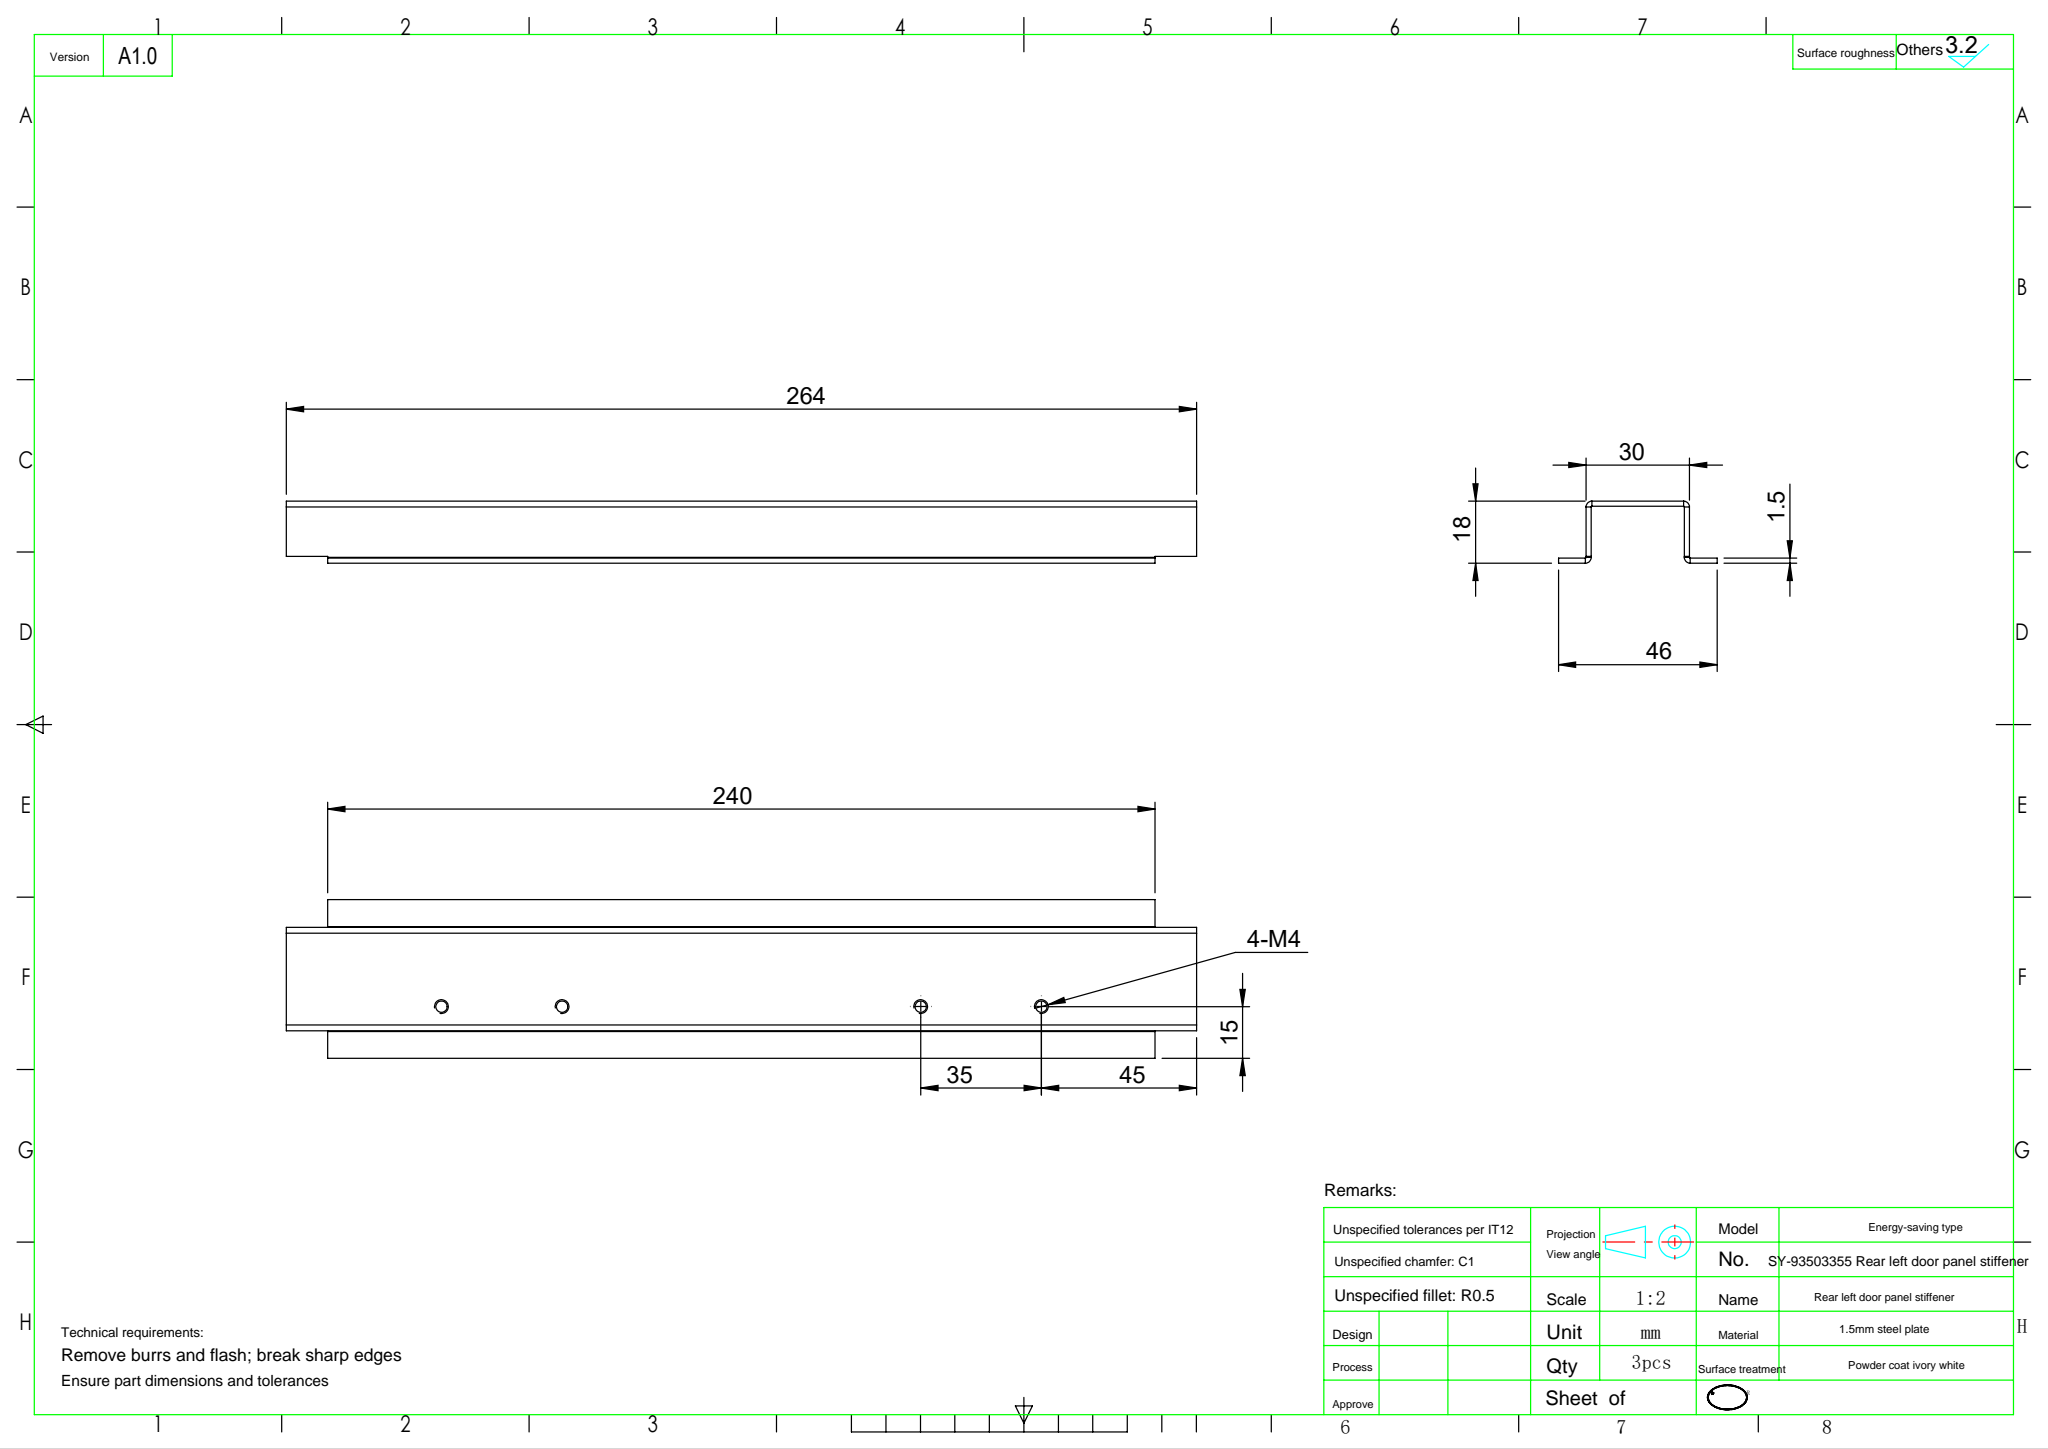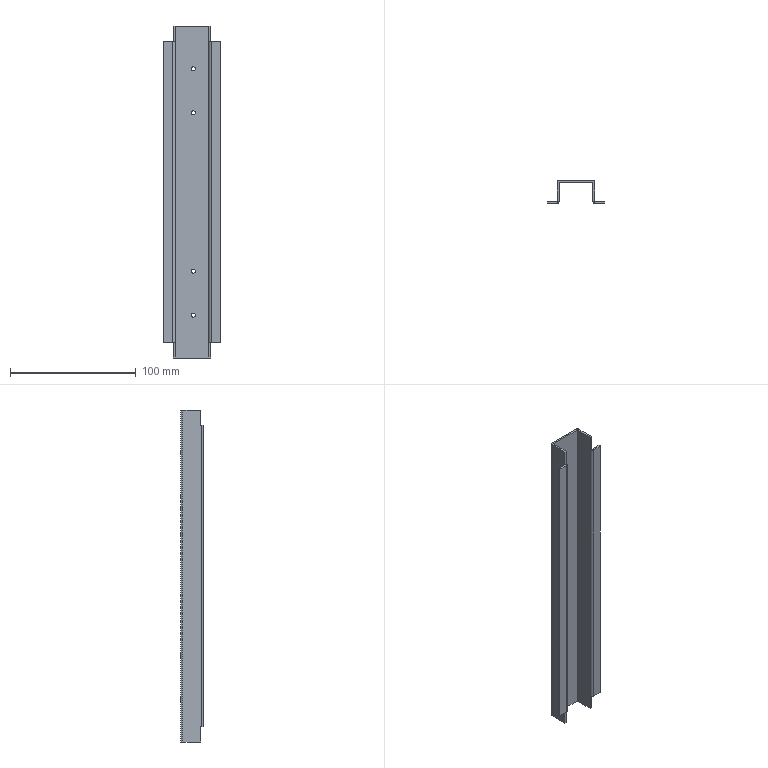Part | SolidWorks | features Cut 1, FlatPattern 1, ICE 1, MirrorPattern 1, SMBaseFlange 1, SheetMetal 1 | 1 solid | 54 faces | box 46 x 18 x 264 mm | volume 29896 mm3 | plane 38 | cylinder 16 | commonest cylinder face diameters 3.3 x8 0.4 x4 3.4 x4